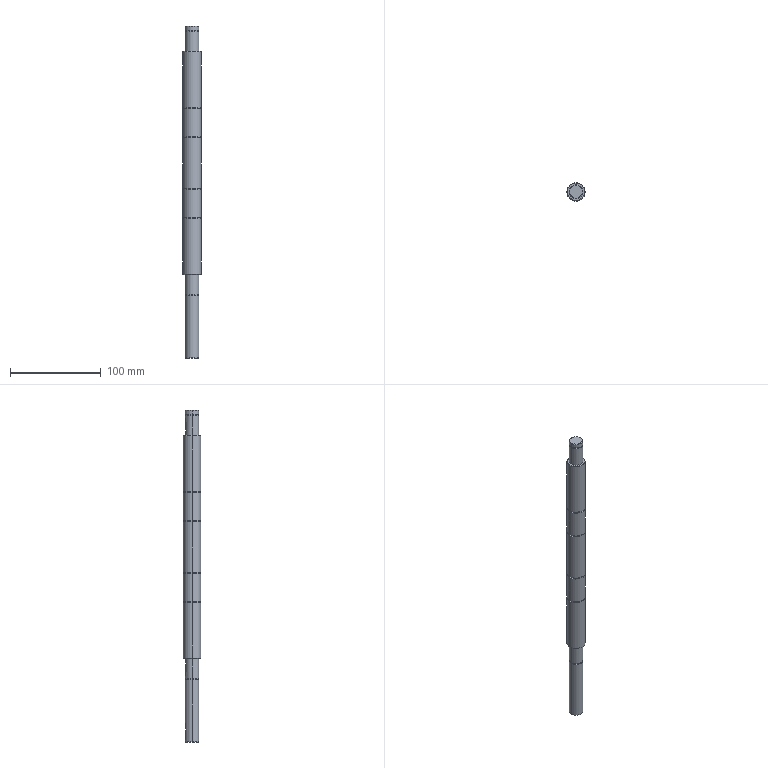Part | STEP file | MYT-A01-P10 | 1 solid | 72 faces | box 20 x 20 x 366.3 mm | volume 97502 mm3 | cylinder 39 | plane 25 | cone 8 | commonest cylinder face diameters 20 x10 5 x9 15 x8 18.8 x8 13.8 x4